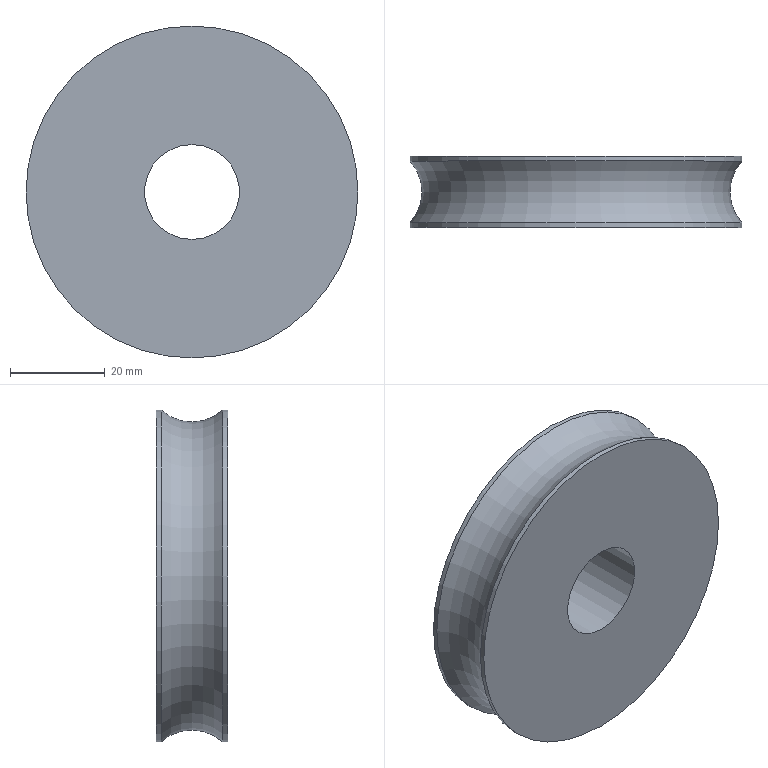Part | NX | features DATUM_CSYS 3, SKETCH 2, Delete Body 1, EXTRUDE 1, SWP104 1 | 1 solid | 6 faces | box 70 x 15 x 70 mm | volume 48198 mm3 | cylinder 3 | plane 2 | torus 1 | commonest cylinder face diameters 70 x2 20 x1
STEP:
#1=CARTESIAN_POINT('',(0.,12.86,21.024));
#2=VERTEX_POINT('',#1);
#3=CARTESIAN_POINT('',(0.,12.86,56.024));
#4=DIRECTION('',(0.,-1.,0.));
#5=DIRECTION('',(0.,0.,-1.));
#6=AXIS2_PLACEMENT_3D('',#3,#4,#5);
#7=CIRCLE('',#6,35.);
#8=EDGE_CURVE('',#2,#2,#7,.T.);
#9=ORIENTED_EDGE('',*,*,#8,.T.);
#10=EDGE_LOOP('',(#9));
#11=FACE_BOUND('',#10,.T.);
#12=CARTESIAN_POINT('',(0.,12.86,46.024));
#13=VERTEX_POINT('',#12);
#14=CARTESIAN_POINT('',(0.,12.86,56.024));
#15=DIRECTION('',(0.,-1.,0.));
#16=DIRECTION('',(0.,0.,-1.));
#17=AXIS2_PLACEMENT_3D('',#14,#15,#16);
#18=CIRCLE('',#17,10.);
#19=EDGE_CURVE('',#13,#13,#18,.T.);
#20=ORIENTED_EDGE('',*,*,#19,.F.);
#21=EDGE_LOOP('',(#20));
#22=FACE_BOUND('',#21,.T.);
#23=CARTESIAN_POINT('',(0.,12.86,46.024));
#24=DIRECTION('',(0.,-1.,0.));
#25=DIRECTION('',(0.,0.,-1.));
#26=AXIS2_PLACEMENT_3D('',#23,#24,#25);
#27=PLANE('',#26);
#28=ADVANCED_FACE('',(#11,#22),#27,.T.);
#29=CARTESIAN_POINT('',(0.,13.86,21.024));
#30=VERTEX_POINT('',#29);
#31=CARTESIAN_POINT('',(0.,13.86,56.024));
#32=DIRECTION('',(0.,-1.,0.));
#33=DIRECTION('',(0.,0.,-1.));
#34=AXIS2_PLACEMENT_3D('',#31,#32,#33);
#35=CIRCLE('',#34,35.);
#36=EDGE_CURVE('',#30,#30,#35,.T.);
#37=ORIENTED_EDGE('',*,*,#36,.T.);
#38=EDGE_LOOP('',(#37));
#39=FACE_BOUND('',#38,.T.);
#40=ORIENTED_EDGE('',*,*,#8,.F.);
#41=EDGE_LOOP('',(#40));
#42=FACE_BOUND('',#41,.T.);
#43=CARTESIAN_POINT('',(0.,27.86,56.024));
#44=DIRECTION('',(0.,-1.,0.));
#45=DIRECTION('',(0.,0.,-1.));
#46=AXIS2_PLACEMENT_3D('',#43,#44,#45);
#47=CYLINDRICAL_SURFACE('',#46,35.);
#48=ADVANCED_FACE('',(#39,#42),#47,.T.);
#49=CARTESIAN_POINT('',(0.,26.86,21.024));
#50=VERTEX_POINT('',#49);
#51=CARTESIAN_POINT('',(0.,26.86,56.024));
#52=DIRECTION('',(0.,-1.,0.));
#53=DIRECTION('',(0.,0.,-1.));
#54=AXIS2_PLACEMENT_3D('',#51,#52,#53);
#55=CIRCLE('',#54,35.);
#56=EDGE_CURVE('',#50,#50,#55,.T.);
#57=ORIENTED_EDGE('',*,*,#56,.T.);
#58=EDGE_LOOP('',(#57));
#59=FACE_BOUND('',#58,.T.);
#60=ORIENTED_EDGE('',*,*,#36,.F.);
#61=EDGE_LOOP('',(#60));
#62=FACE_BOUND('',#61,.T.);
#63=CARTESIAN_POINT('',(0.,20.36,56.024));
#64=DIRECTION('',(0.,-1.,0.));
#65=DIRECTION('',(0.,0.,-1.));
#66=AXIS2_PLACEMENT_3D('',#63,#64,#65);
#67=TOROIDAL_SURFACE('',#66,42.092,9.62);
#68=ADVANCED_FACE('',(#59,#62),#67,.F.);
#69=CARTESIAN_POINT('',(0.,27.86,21.024));
#70=VERTEX_POINT('',#69);
#71=CARTESIAN_POINT('',(0.,27.86,56.024));
#72=DIRECTION('',(0.,-1.,0.));
#73=DIRECTION('',(0.,0.,-1.));
#74=AXIS2_PLACEMENT_3D('',#71,#72,#73);
#75=CIRCLE('',#74,35.);
#76=EDGE_CURVE('',#70,#70,#75,.T.);
#77=ORIENTED_EDGE('',*,*,#76,.T.);
#78=EDGE_LOOP('',(#77));
#79=FACE_BOUND('',#78,.T.);
#80=ORIENTED_EDGE('',*,*,#56,.F.);
#81=EDGE_LOOP('',(#80));
#82=FACE_BOUND('',#81,.T.);
#83=CARTESIAN_POINT('',(0.,27.86,56.024));
#84=DIRECTION('',(0.,-1.,0.));
#85=DIRECTION('',(0.,0.,-1.));
#86=AXIS2_PLACEMENT_3D('',#83,#84,#85);
#87=CYLINDRICAL_SURFACE('',#86,35.);
#88=ADVANCED_FACE('',(#79,#82),#87,.T.);
#89=CARTESIAN_POINT('',(0.,27.86,46.024));
#90=VERTEX_POINT('',#89);
#91=CARTESIAN_POINT('',(0.,27.86,56.024));
#92=DIRECTION('',(0.,-1.,0.));
#93=DIRECTION('',(0.,0.,-1.));
#94=AXIS2_PLACEMENT_3D('',#91,#92,#93);
#95=CIRCLE('',#94,10.);
#96=EDGE_CURVE('',#90,#90,#95,.T.);
#97=ORIENTED_EDGE('',*,*,#96,.T.);
#98=EDGE_LOOP('',(#97));
#99=FACE_BOUND('',#98,.T.);
#100=ORIENTED_EDGE('',*,*,#76,.F.);
#101=EDGE_LOOP('',(#100));
#102=FACE_BOUND('',#101,.T.);
#103=CARTESIAN_POINT('',(0.,27.86,21.024));
#104=DIRECTION('',(0.,1.,0.));
#105=DIRECTION('',(0.,0.,1.));
#106=AXIS2_PLACEMENT_3D('',#103,#104,#105);
#107=PLANE('',#106);
#108=ADVANCED_FACE('',(#99,#102),#107,.T.);
#109=ORIENTED_EDGE('',*,*,#19,.T.);
#110=EDGE_LOOP('',(#109));
#111=FACE_BOUND('',#110,.T.);
#112=ORIENTED_EDGE('',*,*,#96,.F.);
#113=EDGE_LOOP('',(#112));
#114=FACE_BOUND('',#113,.T.);
#115=CARTESIAN_POINT('',(0.,27.86,56.024));
#116=DIRECTION('',(0.,-1.,0.));
#117=DIRECTION('',(0.,0.,-1.));
#118=AXIS2_PLACEMENT_3D('',#115,#116,#117);
#119=CYLINDRICAL_SURFACE('',#118,10.);
#120=ADVANCED_FACE('',(#111,#114),#119,.F.);
#121=CLOSED_SHELL('',(#28,#48,#68,#88,#108,#120));
#122=MANIFOLD_SOLID_BREP('',#121);
#123=(LENGTH_UNIT()NAMED_UNIT(*)SI_UNIT(.MILLI.,.METRE.));
#124=UNCERTAINTY_MEASURE_WITH_UNIT(LENGTH_MEASURE(0.00001),#123,'','');
#125=(NAMED_UNIT(*)PLANE_ANGLE_UNIT()SI_UNIT($,.RADIAN.));
#126=(NAMED_UNIT(*)SI_UNIT($,.STERADIAN.)SOLID_ANGLE_UNIT());
#127=(GEOMETRIC_REPRESENTATION_CONTEXT(3)GLOBAL_UNCERTAINTY_ASSIGNED_CONTEXT((#124))GLOBAL_UNIT_ASSIGNED_CONTEXT((#123,#125,#126))REPRESENTATION_CONTEXT('',''));
#128=ADVANCED_BREP_SHAPE_REPRESENTATION('',(#122),#127);